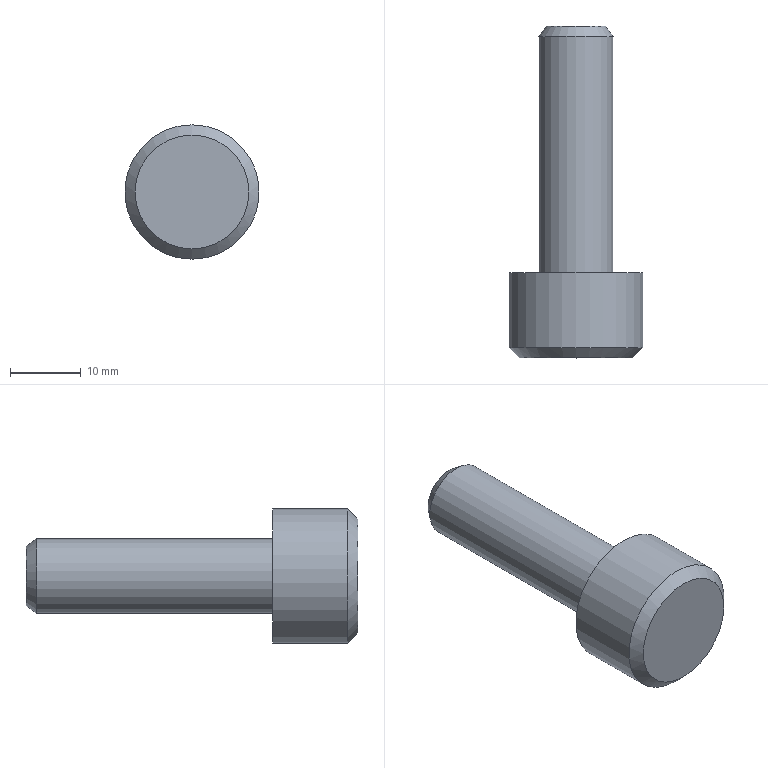Part | STEP file | SCREW-3_id350_x_t | 1 solid | 7 faces | box 18.939 x 46.759 x 18.939 mm | volume 6355 mm3 | plane 3 | cone 2 | cylinder 2 | commonest cylinder face diameters 10.584 x1 18.939 x1
STEP:
#1=CARTESIAN_POINT('',(-92.,-250.,-13.97));
#2=VERTEX_POINT('',#1);
#3=CARTESIAN_POINT('',(-92.,-250.,-22.));
#4=DIRECTION('',(0.,1.,0.));
#5=DIRECTION('',(0.,0.,1.));
#6=AXIS2_PLACEMENT_3D('',#3,#4,#5);
#7=CIRCLE('',#6,8.03);
#8=EDGE_CURVE('',#2,#2,#7,.T.);
#9=ORIENTED_EDGE('',*,*,#8,.F.);
#10=EDGE_LOOP('',(#9));
#11=FACE_OUTER_BOUND('',#10,.T.);
#12=CARTESIAN_POINT('',(-92.,-250.,-22.));
#13=DIRECTION('',(0.,-1.,0.));
#14=DIRECTION('',(0.,0.,-1.));
#15=AXIS2_PLACEMENT_3D('',#12,#13,#14);
#16=PLANE('',#15);
#17=ADVANCED_FACE('',(#11),#16,.T.);
#18=ORIENTED_EDGE('',*,*,#8,.T.);
#19=EDGE_LOOP('',(#18));
#20=FACE_BOUND('',#19,.T.);
#21=CARTESIAN_POINT('',(-92.,-248.57,-31.47));
#22=VERTEX_POINT('',#21);
#23=CARTESIAN_POINT('',(-92.,-248.57,-22.));
#24=DIRECTION('',(0.,1.,0.));
#25=DIRECTION('',(0.,0.,-1.));
#26=AXIS2_PLACEMENT_3D('',#23,#24,#25);
#27=CIRCLE('',#26,9.47);
#28=EDGE_CURVE('',#22,#22,#27,.T.);
#29=ORIENTED_EDGE('',*,*,#28,.F.);
#30=EDGE_LOOP('',(#29));
#31=FACE_BOUND('',#30,.T.);
#32=CARTESIAN_POINT('',(-92.,-248.57,-22.));
#33=DIRECTION('',(0.,1.,0.));
#34=DIRECTION('',(0.,0.,1.));
#35=AXIS2_PLACEMENT_3D('',#32,#33,#34);
#36=CONICAL_SURFACE('',#35,9.47,45.176);
#37=ADVANCED_FACE('',(#20,#31),#36,.T.);
#38=CARTESIAN_POINT('',(-92.,-203.241,-26.178));
#39=VERTEX_POINT('',#38);
#40=CARTESIAN_POINT('',(-92.,-203.241,-22.));
#41=DIRECTION('',(0.,-1.,0.));
#42=DIRECTION('',(0.,0.,-1.));
#43=AXIS2_PLACEMENT_3D('',#40,#41,#42);
#44=CIRCLE('',#43,4.178);
#45=EDGE_CURVE('',#39,#39,#44,.T.);
#46=ORIENTED_EDGE('',*,*,#45,.F.);
#47=EDGE_LOOP('',(#46));
#48=FACE_OUTER_BOUND('',#47,.T.);
#49=CARTESIAN_POINT('',(-92.,-203.241,-22.));
#50=DIRECTION('',(0.,-1.,0.));
#51=DIRECTION('',(0.,0.,-1.));
#52=AXIS2_PLACEMENT_3D('',#49,#50,#51);
#53=PLANE('',#52);
#54=ADVANCED_FACE('',(#48),#53,.F.);
#55=ORIENTED_EDGE('',*,*,#28,.T.);
#56=EDGE_LOOP('',(#55));
#57=FACE_BOUND('',#56,.T.);
#58=CARTESIAN_POINT('',(-92.,-238.,-31.47));
#59=VERTEX_POINT('',#58);
#60=CARTESIAN_POINT('',(-92.,-238.,-22.));
#61=DIRECTION('',(0.,-1.,0.));
#62=DIRECTION('',(0.,0.,-1.));
#63=AXIS2_PLACEMENT_3D('',#60,#61,#62);
#64=CIRCLE('',#63,9.47);
#65=EDGE_CURVE('',#59,#59,#64,.T.);
#66=ORIENTED_EDGE('',*,*,#65,.T.);
#67=EDGE_LOOP('',(#66));
#68=FACE_BOUND('',#67,.T.);
#69=CARTESIAN_POINT('',(-92.,-252.338,-22.));
#70=DIRECTION('',(0.,-1.,0.));
#71=DIRECTION('',(0.,0.,-1.));
#72=AXIS2_PLACEMENT_3D('',#69,#70,#71);
#73=CYLINDRICAL_SURFACE('',#72,9.47);
#74=ADVANCED_FACE('',(#57,#68),#73,.T.);
#75=CARTESIAN_POINT('',(-92.,-204.719,-27.292));
#76=VERTEX_POINT('',#75);
#77=CARTESIAN_POINT('',(-92.,-204.719,-22.));
#78=DIRECTION('',(0.,-1.,0.));
#79=DIRECTION('',(0.,0.,-1.));
#80=AXIS2_PLACEMENT_3D('',#77,#78,#79);
#81=CIRCLE('',#80,5.292);
#82=EDGE_CURVE('',#76,#76,#81,.T.);
#83=ORIENTED_EDGE('',*,*,#82,.F.);
#84=EDGE_LOOP('',(#83));
#85=FACE_BOUND('',#84,.T.);
#86=ORIENTED_EDGE('',*,*,#45,.T.);
#87=EDGE_LOOP('',(#86));
#88=FACE_BOUND('',#87,.T.);
#89=CARTESIAN_POINT('',(-92.,-204.719,-22.));
#90=DIRECTION('',(0.,-1.,0.));
#91=DIRECTION('',(0.,0.,-1.));
#92=AXIS2_PLACEMENT_3D('',#89,#90,#91);
#93=CONICAL_SURFACE('',#92,5.292,37.015);
#94=ADVANCED_FACE('',(#85,#88),#93,.T.);
#95=CARTESIAN_POINT('',(-92.,-238.,-27.292));
#96=VERTEX_POINT('',#95);
#97=CARTESIAN_POINT('',(-92.,-238.,-22.));
#98=DIRECTION('',(0.,1.,0.));
#99=DIRECTION('',(0.,0.,-1.));
#100=AXIS2_PLACEMENT_3D('',#97,#98,#99);
#101=CIRCLE('',#100,5.292);
#102=EDGE_CURVE('',#96,#96,#101,.T.);
#103=ORIENTED_EDGE('',*,*,#102,.F.);
#104=EDGE_LOOP('',(#103));
#105=FACE_BOUND('',#104,.T.);
#106=ORIENTED_EDGE('',*,*,#65,.F.);
#107=EDGE_LOOP('',(#106));
#108=FACE_BOUND('',#107,.T.);
#109=CARTESIAN_POINT('',(-92.,-238.,-22.));
#110=DIRECTION('',(0.,-1.,0.));
#111=DIRECTION('',(0.,0.,-1.));
#112=AXIS2_PLACEMENT_3D('',#109,#110,#111);
#113=PLANE('',#112);
#114=ADVANCED_FACE('',(#105,#108),#113,.F.);
#115=ORIENTED_EDGE('',*,*,#102,.T.);
#116=EDGE_LOOP('',(#115));
#117=FACE_BOUND('',#116,.T.);
#118=ORIENTED_EDGE('',*,*,#82,.T.);
#119=EDGE_LOOP('',(#118));
#120=FACE_BOUND('',#119,.T.);
#121=CARTESIAN_POINT('',(-92.,-252.338,-22.));
#122=DIRECTION('',(0.,-1.,0.));
#123=DIRECTION('',(0.,0.,-1.));
#124=AXIS2_PLACEMENT_3D('',#121,#122,#123);
#125=CYLINDRICAL_SURFACE('',#124,5.292);
#126=ADVANCED_FACE('',(#117,#120),#125,.T.);
#127=CLOSED_SHELL('',(#17,#37,#54,#74,#94,#114,#126));
#128=MANIFOLD_SOLID_BREP('',#127);
#129=(LENGTH_UNIT()NAMED_UNIT(*)SI_UNIT(.MILLI.,.METRE.));
#130=UNCERTAINTY_MEASURE_WITH_UNIT(LENGTH_MEASURE(0.00002),#129,'','');
#131=(NAMED_UNIT(*)PLANE_ANGLE_UNIT()SI_UNIT($,.RADIAN.));
#132=PLANE_ANGLE_MEASURE_WITH_UNIT(PLANE_ANGLE_MEASURE(0.01745),#131);
#133=DIMENSIONAL_EXPONENTS(0.,0.,0.,0.,0.,0.,0.);
#134=(CONVERSION_BASED_UNIT('DEGREE',#132)NAMED_UNIT(#133)PLANE_ANGLE_UNIT());
#135=(NAMED_UNIT(*)SI_UNIT($,.STERADIAN.)SOLID_ANGLE_UNIT());
#136=(GEOMETRIC_REPRESENTATION_CONTEXT(3)GLOBAL_UNCERTAINTY_ASSIGNED_CONTEXT((#130))GLOBAL_UNIT_ASSIGNED_CONTEXT((#129,#134,#135))REPRESENTATION_CONTEXT('',''));
#137=ADVANCED_BREP_SHAPE_REPRESENTATION('',(#128),#136);